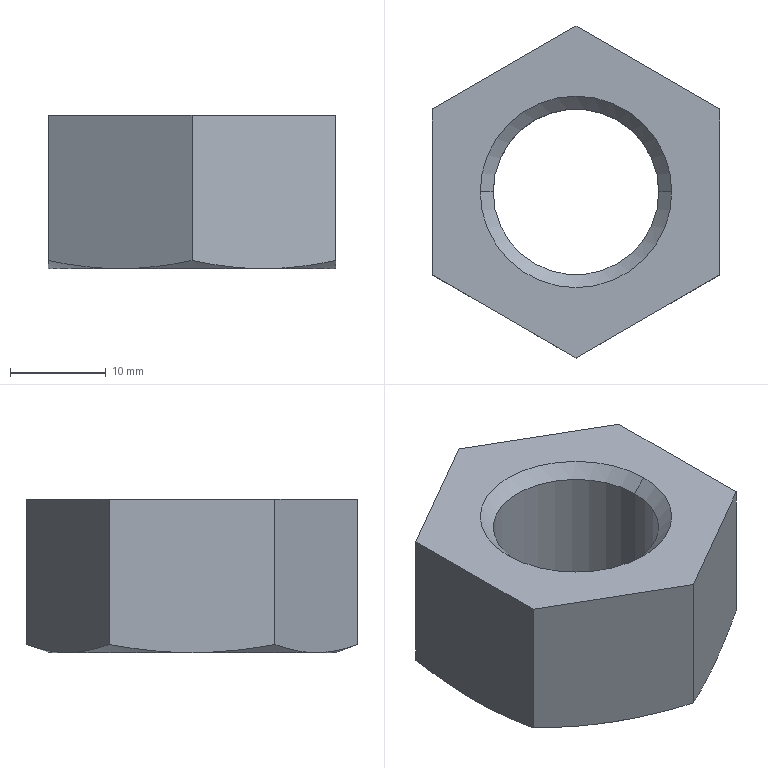Part | SolidWorks | features BaseBody 1 | 1 solid | 20 faces | box 30 x 34.641 x 16 mm | volume 8589 mm3 | cone 10 | plane 8 | cylinder 2 | commonest cylinder face diameters 17.294 x2
STEP:
#1=CARTESIAN_POINT('',(-8.647,0.,1.353));
#2=VERTEX_POINT('',#1);
#3=CARTESIAN_POINT('',(8.647,0.,1.353));
#4=VERTEX_POINT('',#3);
#5=CARTESIAN_POINT('',(0.,0.,1.353));
#6=DIRECTION('',(0.,0.,1.));
#7=DIRECTION('',(1.,0.,0.));
#8=AXIS2_PLACEMENT_3D('',#5,#6,#7);
#9=CIRCLE('',#8,8.647);
#10=EDGE_CURVE('',#2,#4,#9,.T.);
#11=ORIENTED_EDGE('',*,*,#10,.F.);
#12=CARTESIAN_POINT('',(-8.647,0.,14.647));
#13=VERTEX_POINT('',#12);
#14=CARTESIAN_POINT('',(-8.647,0.,0.));
#15=DIRECTION('',(0.,0.,1.));
#16=VECTOR('',#15,1000.);
#17=LINE('',#14,#16);
#18=EDGE_CURVE('',#2,#13,#17,.T.);
#19=ORIENTED_EDGE('',*,*,#18,.T.);
#20=CARTESIAN_POINT('',(8.647,0.,14.647));
#21=VERTEX_POINT('',#20);
#22=CARTESIAN_POINT('',(0.,0.,14.647));
#23=DIRECTION('',(0.,0.,-1.));
#24=DIRECTION('',(1.,0.,0.));
#25=AXIS2_PLACEMENT_3D('',#22,#23,#24);
#26=CIRCLE('',#25,8.647);
#27=EDGE_CURVE('',#21,#13,#26,.T.);
#28=ORIENTED_EDGE('',*,*,#27,.F.);
#29=CARTESIAN_POINT('',(8.647,0.,0.));
#30=DIRECTION('',(0.,0.,1.));
#31=VECTOR('',#30,1000.);
#32=LINE('',#29,#31);
#33=EDGE_CURVE('',#4,#21,#32,.T.);
#34=ORIENTED_EDGE('',*,*,#33,.F.);
#35=EDGE_LOOP('',(#11,#19,#28,#34));
#36=FACE_OUTER_BOUND('',#35,.T.);
#37=CARTESIAN_POINT('',(0.,0.,0.));
#38=DIRECTION('',(0.,0.,1.));
#39=DIRECTION('',(1.,0.,0.));
#40=AXIS2_PLACEMENT_3D('',#37,#38,#39);
#41=CYLINDRICAL_SURFACE('',#40,8.647);
#42=ADVANCED_FACE('',(#36),#41,.F.);
#43=ORIENTED_EDGE('',*,*,#27,.T.);
#44=CARTESIAN_POINT('',(-10.,0.,16.));
#45=VERTEX_POINT('',#44);
#46=CARTESIAN_POINT('',(-10.,0.,16.));
#47=DIRECTION('',(-0.7071,0.,0.7071));
#48=VECTOR('',#47,1000.);
#49=LINE('',#46,#48);
#50=EDGE_CURVE('',#13,#45,#49,.T.);
#51=ORIENTED_EDGE('',*,*,#50,.T.);
#52=CARTESIAN_POINT('',(10.,0.,16.));
#53=VERTEX_POINT('',#52);
#54=CARTESIAN_POINT('',(0.,0.,16.));
#55=DIRECTION('',(0.,0.,-1.));
#56=DIRECTION('',(1.,0.,0.));
#57=AXIS2_PLACEMENT_3D('',#54,#55,#56);
#58=CIRCLE('',#57,10.);
#59=EDGE_CURVE('',#53,#45,#58,.T.);
#60=ORIENTED_EDGE('',*,*,#59,.F.);
#61=CARTESIAN_POINT('',(10.,0.,16.));
#62=DIRECTION('',(0.7071,0.,0.7071));
#63=VECTOR('',#62,1000.);
#64=LINE('',#61,#63);
#65=EDGE_CURVE('',#21,#53,#64,.T.);
#66=ORIENTED_EDGE('',*,*,#65,.F.);
#67=EDGE_LOOP('',(#43,#51,#60,#66));
#68=FACE_OUTER_BOUND('',#67,.T.);
#69=CARTESIAN_POINT('',(0.,0.,16.));
#70=DIRECTION('',(0.,0.,1.));
#71=DIRECTION('',(1.,0.,0.));
#72=AXIS2_PLACEMENT_3D('',#69,#70,#71);
#73=CONICAL_SURFACE('',#72,10.,0.7854);
#74=ADVANCED_FACE('',(#68),#73,.F.);
#75=ORIENTED_EDGE('',*,*,#10,.T.);
#76=CARTESIAN_POINT('',(10.,0.,0.));
#77=VERTEX_POINT('',#76);
#78=CARTESIAN_POINT('',(10.,0.,0.));
#79=DIRECTION('',(0.7071,0.,-0.7071));
#80=VECTOR('',#79,1000.);
#81=LINE('',#78,#80);
#82=EDGE_CURVE('',#4,#77,#81,.T.);
#83=ORIENTED_EDGE('',*,*,#82,.T.);
#84=CARTESIAN_POINT('',(-10.,0.,0.));
#85=VERTEX_POINT('',#84);
#86=CARTESIAN_POINT('',(0.,0.,0.));
#87=DIRECTION('',(0.,0.,1.));
#88=DIRECTION('',(-1.,0.,0.));
#89=AXIS2_PLACEMENT_3D('',#86,#87,#88);
#90=CIRCLE('',#89,10.);
#91=EDGE_CURVE('',#85,#77,#90,.T.);
#92=ORIENTED_EDGE('',*,*,#91,.F.);
#93=CARTESIAN_POINT('',(-10.,0.,0.));
#94=DIRECTION('',(-0.7071,0.,-0.7071));
#95=VECTOR('',#94,1000.);
#96=LINE('',#93,#95);
#97=EDGE_CURVE('',#2,#85,#96,.T.);
#98=ORIENTED_EDGE('',*,*,#97,.F.);
#99=EDGE_LOOP('',(#75,#83,#92,#98));
#100=FACE_OUTER_BOUND('',#99,.T.);
#101=CARTESIAN_POINT('',(0.,0.,0.));
#102=DIRECTION('',(0.,0.,-1.));
#103=DIRECTION('',(-1.,0.,0.));
#104=AXIS2_PLACEMENT_3D('',#101,#102,#103);
#105=CONICAL_SURFACE('',#104,10.,0.7854);
#106=ADVANCED_FACE('',(#100),#105,.F.);
#107=ORIENTED_EDGE('',*,*,#18,.F.);
#108=CARTESIAN_POINT('',(0.,0.,1.353));
#109=DIRECTION('',(0.,0.,1.));
#110=DIRECTION('',(1.,0.,0.));
#111=AXIS2_PLACEMENT_3D('',#108,#109,#110);
#112=CIRCLE('',#111,8.647);
#113=EDGE_CURVE('',#4,#2,#112,.T.);
#114=ORIENTED_EDGE('',*,*,#113,.F.);
#115=ORIENTED_EDGE('',*,*,#33,.T.);
#116=CARTESIAN_POINT('',(0.,0.,14.647));
#117=DIRECTION('',(0.,0.,-1.));
#118=DIRECTION('',(1.,0.,0.));
#119=AXIS2_PLACEMENT_3D('',#116,#117,#118);
#120=CIRCLE('',#119,8.647);
#121=EDGE_CURVE('',#13,#21,#120,.T.);
#122=ORIENTED_EDGE('',*,*,#121,.F.);
#123=EDGE_LOOP('',(#107,#114,#115,#122));
#124=FACE_OUTER_BOUND('',#123,.T.);
#125=CARTESIAN_POINT('',(0.,0.,0.));
#126=DIRECTION('',(0.,0.,1.));
#127=DIRECTION('',(1.,0.,0.));
#128=AXIS2_PLACEMENT_3D('',#125,#126,#127);
#129=CYLINDRICAL_SURFACE('',#128,8.647);
#130=ADVANCED_FACE('',(#124),#129,.F.);
#131=ORIENTED_EDGE('',*,*,#50,.F.);
#132=ORIENTED_EDGE('',*,*,#121,.T.);
#133=ORIENTED_EDGE('',*,*,#65,.T.);
#134=CARTESIAN_POINT('',(0.,0.,16.));
#135=DIRECTION('',(0.,0.,-1.));
#136=DIRECTION('',(1.,0.,0.));
#137=AXIS2_PLACEMENT_3D('',#134,#135,#136);
#138=CIRCLE('',#137,10.);
#139=EDGE_CURVE('',#45,#53,#138,.T.);
#140=ORIENTED_EDGE('',*,*,#139,.F.);
#141=EDGE_LOOP('',(#131,#132,#133,#140));
#142=FACE_OUTER_BOUND('',#141,.T.);
#143=CARTESIAN_POINT('',(0.,0.,16.));
#144=DIRECTION('',(0.,0.,1.));
#145=DIRECTION('',(1.,0.,0.));
#146=AXIS2_PLACEMENT_3D('',#143,#144,#145);
#147=CONICAL_SURFACE('',#146,10.,0.7854);
#148=ADVANCED_FACE('',(#142),#147,.F.);
#149=ORIENTED_EDGE('',*,*,#82,.F.);
#150=ORIENTED_EDGE('',*,*,#113,.T.);
#151=ORIENTED_EDGE('',*,*,#97,.T.);
#152=CARTESIAN_POINT('',(0.,0.,0.));
#153=DIRECTION('',(0.,0.,1.));
#154=DIRECTION('',(-1.,0.,0.));
#155=AXIS2_PLACEMENT_3D('',#152,#153,#154);
#156=CIRCLE('',#155,10.);
#157=EDGE_CURVE('',#77,#85,#156,.T.);
#158=ORIENTED_EDGE('',*,*,#157,.F.);
#159=EDGE_LOOP('',(#149,#150,#151,#158));
#160=FACE_OUTER_BOUND('',#159,.T.);
#161=CARTESIAN_POINT('',(0.,0.,0.));
#162=DIRECTION('',(0.,0.,-1.));
#163=DIRECTION('',(-1.,0.,0.));
#164=AXIS2_PLACEMENT_3D('',#161,#162,#163);
#165=CONICAL_SURFACE('',#164,10.,0.7854);
#166=ADVANCED_FACE('',(#160),#165,.F.);
#167=ORIENTED_EDGE('',*,*,#59,.T.);
#168=ORIENTED_EDGE('',*,*,#139,.T.);
#169=EDGE_LOOP('',(#167,#168));
#170=FACE_BOUND('',#169,.T.);
#171=CARTESIAN_POINT('',(15.,-8.66,16.));
#172=VERTEX_POINT('',#171);
#173=CARTESIAN_POINT('',(15.,8.66,16.));
#174=VERTEX_POINT('',#173);
#175=CARTESIAN_POINT('',(15.,0.,16.));
#176=DIRECTION('',(0.,1.,0.));
#177=VECTOR('',#176,1000.);
#178=LINE('',#175,#177);
#179=EDGE_CURVE('',#172,#174,#178,.T.);
#180=ORIENTED_EDGE('',*,*,#179,.T.);
#181=CARTESIAN_POINT('',(0.,17.321,16.));
#182=VERTEX_POINT('',#181);
#183=CARTESIAN_POINT('',(15.,8.66,16.));
#184=DIRECTION('',(-0.866,0.5,0.));
#185=VECTOR('',#184,1000.);
#186=LINE('',#183,#185);
#187=EDGE_CURVE('',#174,#182,#186,.T.);
#188=ORIENTED_EDGE('',*,*,#187,.T.);
#189=CARTESIAN_POINT('',(-15.,8.66,16.));
#190=VERTEX_POINT('',#189);
#191=CARTESIAN_POINT('',(0.,17.321,16.));
#192=DIRECTION('',(-0.866,-0.5,0.));
#193=VECTOR('',#192,1000.);
#194=LINE('',#191,#193);
#195=EDGE_CURVE('',#182,#190,#194,.T.);
#196=ORIENTED_EDGE('',*,*,#195,.T.);
#197=CARTESIAN_POINT('',(-15.,-8.66,16.));
#198=VERTEX_POINT('',#197);
#199=CARTESIAN_POINT('',(-15.,0.,16.));
#200=DIRECTION('',(0.,-1.,0.));
#201=VECTOR('',#200,1000.);
#202=LINE('',#199,#201);
#203=EDGE_CURVE('',#190,#198,#202,.T.);
#204=ORIENTED_EDGE('',*,*,#203,.T.);
#205=CARTESIAN_POINT('',(0.,-17.321,16.));
#206=VERTEX_POINT('',#205);
#207=CARTESIAN_POINT('',(-15.,-8.66,16.));
#208=DIRECTION('',(0.866,-0.5,0.));
#209=VECTOR('',#208,1000.);
#210=LINE('',#207,#209);
#211=EDGE_CURVE('',#198,#206,#210,.T.);
#212=ORIENTED_EDGE('',*,*,#211,.T.);
#213=CARTESIAN_POINT('',(0.,-17.321,16.));
#214=DIRECTION('',(0.866,0.5,0.));
#215=VECTOR('',#214,1000.);
#216=LINE('',#213,#215);
#217=EDGE_CURVE('',#206,#172,#216,.T.);
#218=ORIENTED_EDGE('',*,*,#217,.T.);
#219=EDGE_LOOP('',(#180,#188,#196,#204,#212,#218));
#220=FACE_OUTER_BOUND('',#219,.T.);
#221=CARTESIAN_POINT('',(0.,0.,16.));
#222=DIRECTION('',(0.,0.,1.));
#223=DIRECTION('',(1.,0.,0.));
#224=AXIS2_PLACEMENT_3D('',#221,#222,#223);
#225=PLANE('',#224);
#226=ADVANCED_FACE('',(#170,#220),#225,.T.);
#227=ORIENTED_EDGE('',*,*,#91,.T.);
#228=ORIENTED_EDGE('',*,*,#157,.T.);
#229=EDGE_LOOP('',(#227,#228));
#230=FACE_BOUND('',#229,.T.);
#231=CARTESIAN_POINT('',(-7.5,-12.99,0.));
#232=VERTEX_POINT('',#231);
#233=CARTESIAN_POINT('',(7.5,-12.99,0.));
#234=VERTEX_POINT('',#233);
#235=CARTESIAN_POINT('',(0.,0.,0.));
#236=DIRECTION('',(0.,0.,1.));
#237=DIRECTION('',(1.,0.,0.));
#238=AXIS2_PLACEMENT_3D('',#235,#236,#237);
#239=CIRCLE('',#238,15.);
#240=EDGE_CURVE('',#232,#234,#239,.T.);
#241=ORIENTED_EDGE('',*,*,#240,.F.);
#242=CARTESIAN_POINT('',(-15.,0.,0.));
#243=VERTEX_POINT('',#242);
#244=CARTESIAN_POINT('',(0.,0.,0.));
#245=DIRECTION('',(0.,0.,1.));
#246=DIRECTION('',(0.,-1.,0.));
#247=AXIS2_PLACEMENT_3D('',#244,#245,#246);
#248=CIRCLE('',#247,15.);
#249=EDGE_CURVE('',#243,#232,#248,.T.);
#250=ORIENTED_EDGE('',*,*,#249,.F.);
#251=CARTESIAN_POINT('',(-7.5,12.99,0.));
#252=VERTEX_POINT('',#251);
#253=CARTESIAN_POINT('',(0.,0.,0.));
#254=DIRECTION('',(0.,0.,1.));
#255=DIRECTION('',(0.,-1.,0.));
#256=AXIS2_PLACEMENT_3D('',#253,#254,#255);
#257=CIRCLE('',#256,15.);
#258=EDGE_CURVE('',#252,#243,#257,.T.);
#259=ORIENTED_EDGE('',*,*,#258,.F.);
#260=CARTESIAN_POINT('',(7.5,12.99,0.));
#261=VERTEX_POINT('',#260);
#262=CARTESIAN_POINT('',(0.,0.,0.));
#263=DIRECTION('',(0.,0.,1.));
#264=DIRECTION('',(1.,0.,0.));
#265=AXIS2_PLACEMENT_3D('',#262,#263,#264);
#266=CIRCLE('',#265,15.);
#267=EDGE_CURVE('',#261,#252,#266,.T.);
#268=ORIENTED_EDGE('',*,*,#267,.F.);
#269=CARTESIAN_POINT('',(15.,0.,0.));
#270=VERTEX_POINT('',#269);
#271=CARTESIAN_POINT('',(0.,0.,0.));
#272=DIRECTION('',(0.,0.,1.));
#273=DIRECTION('',(0.,-1.,0.));
#274=AXIS2_PLACEMENT_3D('',#271,#272,#273);
#275=CIRCLE('',#274,15.);
#276=EDGE_CURVE('',#270,#261,#275,.T.);
#277=ORIENTED_EDGE('',*,*,#276,.F.);
#278=CARTESIAN_POINT('',(0.,0.,0.));
#279=DIRECTION('',(0.,0.,1.));
#280=DIRECTION('',(1.,0.,0.));
#281=AXIS2_PLACEMENT_3D('',#278,#279,#280);
#282=CIRCLE('',#281,15.);
#283=EDGE_CURVE('',#234,#270,#282,.T.);
#284=ORIENTED_EDGE('',*,*,#283,.F.);
#285=EDGE_LOOP('',(#241,#250,#259,#268,#277,#284));
#286=FACE_OUTER_BOUND('',#285,.T.);
#287=CARTESIAN_POINT('',(0.,0.,0.));
#288=DIRECTION('',(0.,0.,1.));
#289=DIRECTION('',(1.,0.,0.));
#290=AXIS2_PLACEMENT_3D('',#287,#288,#289);
#291=PLANE('',#290);
#292=ADVANCED_FACE('',(#230,#286),#291,.F.);
#293=CARTESIAN_POINT('',(15.,8.66,0.8446));
#294=VERTEX_POINT('',#293);
#295=CARTESIAN_POINT('',(7.5,12.99,0.));
#296=CARTESIAN_POINT('',(8.762,12.262,0.));
#297=CARTESIAN_POINT('',(10.017,11.537,0.07863));
#298=CARTESIAN_POINT('',(12.516,10.094,0.3711));
#299=CARTESIAN_POINT('',(13.76,9.376,0.584));
#300=CARTESIAN_POINT('',(15.,8.66,0.8446));
#301=B_SPLINE_CURVE_WITH_KNOTS('',3,(#295,#296,#297,#298,#299,#300),.UNSPECIFIED.,.F.,.F.,(4,2,4),(0.,0.004351,0.008701),.UNSPECIFIED.);
#302=EDGE_CURVE('',#261,#294,#301,.T.);
#303=ORIENTED_EDGE('',*,*,#302,.F.);
#304=CARTESIAN_POINT('',(0.,17.321,0.8446));
#305=VERTEX_POINT('',#304);
#306=CARTESIAN_POINT('',(0.,17.321,0.8446));
#307=CARTESIAN_POINT('',(1.24,16.605,0.584));
#308=CARTESIAN_POINT('',(2.484,15.886,0.3711));
#309=CARTESIAN_POINT('',(4.983,14.444,0.07863));
#310=CARTESIAN_POINT('',(6.238,13.719,0.));
#311=CARTESIAN_POINT('',(7.5,12.99,0.));
#312=B_SPLINE_CURVE_WITH_KNOTS('',3,(#306,#307,#308,#309,#310,#311),.UNSPECIFIED.,.F.,.F.,(4,2,4),(0.,0.004351,0.008701),.UNSPECIFIED.);
#313=EDGE_CURVE('',#305,#261,#312,.T.);
#314=ORIENTED_EDGE('',*,*,#313,.F.);
#315=CARTESIAN_POINT('',(0.,17.321,16.));
#316=DIRECTION('',(0.,0.,-1.));
#317=VECTOR('',#316,1000.);
#318=LINE('',#315,#317);
#319=EDGE_CURVE('',#182,#305,#318,.T.);
#320=ORIENTED_EDGE('',*,*,#319,.F.);
#321=ORIENTED_EDGE('',*,*,#187,.F.);
#322=CARTESIAN_POINT('',(15.,8.66,16.));
#323=DIRECTION('',(0.,0.,1.));
#324=VECTOR('',#323,1000.);
#325=LINE('',#322,#324);
#326=EDGE_CURVE('',#294,#174,#325,.T.);
#327=ORIENTED_EDGE('',*,*,#326,.F.);
#328=EDGE_LOOP('',(#303,#314,#320,#321,#327));
#329=FACE_OUTER_BOUND('',#328,.T.);
#330=CARTESIAN_POINT('',(15.,8.66,16.));
#331=DIRECTION('',(-0.5,-0.866,0.));
#332=DIRECTION('',(0.866,-0.5,0.));
#333=AXIS2_PLACEMENT_3D('',#330,#331,#332);
#334=PLANE('',#333);
#335=ADVANCED_FACE('',(#329),#334,.F.);
#336=CARTESIAN_POINT('',(15.,-8.66,0.8446));
#337=VERTEX_POINT('',#336);
#338=CARTESIAN_POINT('',(15.,0.,0.));
#339=CARTESIAN_POINT('',(15.,-1.457,0.));
#340=CARTESIAN_POINT('',(15.,-2.907,0.07863));
#341=CARTESIAN_POINT('',(15.,-5.792,0.3711));
#342=CARTESIAN_POINT('',(15.,-7.229,0.584));
#343=CARTESIAN_POINT('',(15.,-8.66,0.8446));
#344=B_SPLINE_CURVE_WITH_KNOTS('',3,(#338,#339,#340,#341,#342,#343),.UNSPECIFIED.,.F.,.F.,(4,2,4),(0.,0.004351,0.008701),.UNSPECIFIED.);
#345=EDGE_CURVE('',#270,#337,#344,.T.);
#346=ORIENTED_EDGE('',*,*,#345,.F.);
#347=CARTESIAN_POINT('',(15.,8.66,0.8446));
#348=CARTESIAN_POINT('',(15.,7.229,0.584));
#349=CARTESIAN_POINT('',(15.,5.792,0.3711));
#350=CARTESIAN_POINT('',(15.,2.907,0.07863));
#351=CARTESIAN_POINT('',(15.,1.457,0.));
#352=CARTESIAN_POINT('',(15.,0.,0.));
#353=B_SPLINE_CURVE_WITH_KNOTS('',3,(#347,#348,#349,#350,#351,#352),.UNSPECIFIED.,.F.,.F.,(4,2,4),(0.,0.004351,0.008701),.UNSPECIFIED.);
#354=EDGE_CURVE('',#294,#270,#353,.T.);
#355=ORIENTED_EDGE('',*,*,#354,.F.);
#356=ORIENTED_EDGE('',*,*,#326,.T.);
#357=ORIENTED_EDGE('',*,*,#179,.F.);
#358=CARTESIAN_POINT('',(15.,-8.66,16.));
#359=DIRECTION('',(0.,0.,1.));
#360=VECTOR('',#359,1000.);
#361=LINE('',#358,#360);
#362=EDGE_CURVE('',#337,#172,#361,.T.);
#363=ORIENTED_EDGE('',*,*,#362,.F.);
#364=EDGE_LOOP('',(#346,#355,#356,#357,#363));
#365=FACE_OUTER_BOUND('',#364,.T.);
#366=CARTESIAN_POINT('',(15.,-8.66,16.));
#367=DIRECTION('',(-1.,0.,0.));
#368=DIRECTION('',(0.,0.,1.));
#369=AXIS2_PLACEMENT_3D('',#366,#367,#368);
#370=PLANE('',#369);
#371=ADVANCED_FACE('',(#365),#370,.F.);
#372=CARTESIAN_POINT('',(0.,-17.321,0.8446));
#373=VERTEX_POINT('',#372);
#374=CARTESIAN_POINT('',(7.5,-12.99,0.));
#375=CARTESIAN_POINT('',(6.238,-13.719,0.));
#376=CARTESIAN_POINT('',(4.983,-14.444,0.07863));
#377=CARTESIAN_POINT('',(2.484,-15.886,0.3711));
#378=CARTESIAN_POINT('',(1.24,-16.605,0.584));
#379=CARTESIAN_POINT('',(0.,-17.321,0.8446));
#380=B_SPLINE_CURVE_WITH_KNOTS('',3,(#374,#375,#376,#377,#378,#379),.UNSPECIFIED.,.F.,.F.,(4,2,4),(0.,0.004351,0.008701),.UNSPECIFIED.);
#381=EDGE_CURVE('',#234,#373,#380,.T.);
#382=ORIENTED_EDGE('',*,*,#381,.F.);
#383=CARTESIAN_POINT('',(15.,-8.66,0.8446));
#384=CARTESIAN_POINT('',(13.76,-9.376,0.584));
#385=CARTESIAN_POINT('',(12.516,-10.094,0.3711));
#386=CARTESIAN_POINT('',(10.017,-11.537,0.07863));
#387=CARTESIAN_POINT('',(8.762,-12.262,0.));
#388=CARTESIAN_POINT('',(7.5,-12.99,0.));
#389=B_SPLINE_CURVE_WITH_KNOTS('',3,(#383,#384,#385,#386,#387,#388),.UNSPECIFIED.,.F.,.F.,(4,2,4),(0.,0.004351,0.008701),.UNSPECIFIED.);
#390=EDGE_CURVE('',#337,#234,#389,.T.);
#391=ORIENTED_EDGE('',*,*,#390,.F.);
#392=ORIENTED_EDGE('',*,*,#362,.T.);
#393=ORIENTED_EDGE('',*,*,#217,.F.);
#394=CARTESIAN_POINT('',(0.,-17.321,16.));
#395=DIRECTION('',(0.,0.,1.));
#396=VECTOR('',#395,1000.);
#397=LINE('',#394,#396);
#398=EDGE_CURVE('',#373,#206,#397,.T.);
#399=ORIENTED_EDGE('',*,*,#398,.F.);
#400=EDGE_LOOP('',(#382,#391,#392,#393,#399));
#401=FACE_OUTER_BOUND('',#400,.T.);
#402=CARTESIAN_POINT('',(0.,-17.321,16.));
#403=DIRECTION('',(-0.5,0.866,0.));
#404=DIRECTION('',(-0.866,-0.5,0.));
#405=AXIS2_PLACEMENT_3D('',#402,#403,#404);
#406=PLANE('',#405);
#407=ADVANCED_FACE('',(#401),#406,.F.);
#408=CARTESIAN_POINT('',(-15.,-8.66,0.8446));
#409=VERTEX_POINT('',#408);
#410=CARTESIAN_POINT('',(-7.5,-12.99,0.));
#411=CARTESIAN_POINT('',(-8.762,-12.262,0.));
#412=CARTESIAN_POINT('',(-10.017,-11.537,0.07863));
#413=CARTESIAN_POINT('',(-12.516,-10.094,0.3711));
#414=CARTESIAN_POINT('',(-13.76,-9.376,0.584));
#415=CARTESIAN_POINT('',(-15.,-8.66,0.8446));
#416=B_SPLINE_CURVE_WITH_KNOTS('',3,(#410,#411,#412,#413,#414,#415),.UNSPECIFIED.,.F.,.F.,(4,2,4),(0.,0.004351,0.008701),.UNSPECIFIED.);
#417=EDGE_CURVE('',#232,#409,#416,.T.);
#418=ORIENTED_EDGE('',*,*,#417,.F.);
#419=CARTESIAN_POINT('',(0.,-17.321,0.8446));
#420=CARTESIAN_POINT('',(-1.24,-16.605,0.584));
#421=CARTESIAN_POINT('',(-2.484,-15.886,0.3711));
#422=CARTESIAN_POINT('',(-4.983,-14.444,0.07863));
#423=CARTESIAN_POINT('',(-6.238,-13.719,0.));
#424=CARTESIAN_POINT('',(-7.5,-12.99,0.));
#425=B_SPLINE_CURVE_WITH_KNOTS('',3,(#419,#420,#421,#422,#423,#424),.UNSPECIFIED.,.F.,.F.,(4,2,4),(0.,0.004351,0.008701),.UNSPECIFIED.);
#426=EDGE_CURVE('',#373,#232,#425,.T.);
#427=ORIENTED_EDGE('',*,*,#426,.F.);
#428=ORIENTED_EDGE('',*,*,#398,.T.);
#429=ORIENTED_EDGE('',*,*,#211,.F.);
#430=CARTESIAN_POINT('',(-15.,-8.66,16.));
#431=DIRECTION('',(0.,0.,1.));
#432=VECTOR('',#431,1000.);
#433=LINE('',#430,#432);
#434=EDGE_CURVE('',#409,#198,#433,.T.);
#435=ORIENTED_EDGE('',*,*,#434,.F.);
#436=EDGE_LOOP('',(#418,#427,#428,#429,#435));
#437=FACE_OUTER_BOUND('',#436,.T.);
#438=CARTESIAN_POINT('',(-15.,-8.66,16.));
#439=DIRECTION('',(0.5,0.866,0.));
#440=DIRECTION('',(-0.866,0.5,0.));
#441=AXIS2_PLACEMENT_3D('',#438,#439,#440);
#442=PLANE('',#441);
#443=ADVANCED_FACE('',(#437),#442,.F.);
#444=CARTESIAN_POINT('',(-15.,8.66,0.8446));
#445=VERTEX_POINT('',#444);
#446=CARTESIAN_POINT('',(-15.,0.,0.));
#447=CARTESIAN_POINT('',(-15.,1.457,0.));
#448=CARTESIAN_POINT('',(-15.,2.907,0.07863));
#449=CARTESIAN_POINT('',(-15.,5.792,0.3711));
#450=CARTESIAN_POINT('',(-15.,7.229,0.584));
#451=CARTESIAN_POINT('',(-15.,8.66,0.8446));
#452=B_SPLINE_CURVE_WITH_KNOTS('',3,(#446,#447,#448,#449,#450,#451),.UNSPECIFIED.,.F.,.F.,(4,2,4),(0.,0.004351,0.008701),.UNSPECIFIED.);
#453=EDGE_CURVE('',#243,#445,#452,.T.);
#454=ORIENTED_EDGE('',*,*,#453,.F.);
#455=CARTESIAN_POINT('',(-15.,-8.66,0.8446));
#456=CARTESIAN_POINT('',(-15.,-7.229,0.584));
#457=CARTESIAN_POINT('',(-15.,-5.792,0.3711));
#458=CARTESIAN_POINT('',(-15.,-2.907,0.07863));
#459=CARTESIAN_POINT('',(-15.,-1.457,0.));
#460=CARTESIAN_POINT('',(-15.,0.,0.));
#461=B_SPLINE_CURVE_WITH_KNOTS('',3,(#455,#456,#457,#458,#459,#460),.UNSPECIFIED.,.F.,.F.,(4,2,4),(0.,0.004351,0.008701),.UNSPECIFIED.);
#462=EDGE_CURVE('',#409,#243,#461,.T.);
#463=ORIENTED_EDGE('',*,*,#462,.F.);
#464=ORIENTED_EDGE('',*,*,#434,.T.);
#465=ORIENTED_EDGE('',*,*,#203,.F.);
#466=CARTESIAN_POINT('',(-15.,8.66,16.));
#467=DIRECTION('',(0.,0.,1.));
#468=VECTOR('',#467,1000.);
#469=LINE('',#466,#468);
#470=EDGE_CURVE('',#445,#190,#469,.T.);
#471=ORIENTED_EDGE('',*,*,#470,.F.);
#472=EDGE_LOOP('',(#454,#463,#464,#465,#471));
#473=FACE_OUTER_BOUND('',#472,.T.);
#474=CARTESIAN_POINT('',(-15.,8.66,16.));
#475=DIRECTION('',(1.,0.,0.));
#476=DIRECTION('',(0.,0.,-1.));
#477=AXIS2_PLACEMENT_3D('',#474,#475,#476);
#478=PLANE('',#477);
#479=ADVANCED_FACE('',(#473),#478,.F.);
#480=CARTESIAN_POINT('',(-7.5,12.99,0.));
#481=CARTESIAN_POINT('',(-6.238,13.719,0.));
#482=CARTESIAN_POINT('',(-4.983,14.444,0.07863));
#483=CARTESIAN_POINT('',(-2.484,15.886,0.3711));
#484=CARTESIAN_POINT('',(-1.24,16.605,0.584));
#485=CARTESIAN_POINT('',(0.,17.321,0.8446));
#486=B_SPLINE_CURVE_WITH_KNOTS('',3,(#480,#481,#482,#483,#484,#485),.UNSPECIFIED.,.F.,.F.,(4,2,4),(0.,0.004351,0.008701),.UNSPECIFIED.);
#487=EDGE_CURVE('',#252,#305,#486,.T.);
#488=ORIENTED_EDGE('',*,*,#487,.F.);
#489=CARTESIAN_POINT('',(-15.,8.66,0.8446));
#490=CARTESIAN_POINT('',(-13.76,9.376,0.584));
#491=CARTESIAN_POINT('',(-12.516,10.094,0.3711));
#492=CARTESIAN_POINT('',(-10.017,11.537,0.07863));
#493=CARTESIAN_POINT('',(-8.762,12.262,0.));
#494=CARTESIAN_POINT('',(-7.5,12.99,0.));
#495=B_SPLINE_CURVE_WITH_KNOTS('',3,(#489,#490,#491,#492,#493,#494),.UNSPECIFIED.,.F.,.F.,(4,2,4),(0.,0.004351,0.008701),.UNSPECIFIED.);
#496=EDGE_CURVE('',#445,#252,#495,.T.);
#497=ORIENTED_EDGE('',*,*,#496,.F.);
#498=ORIENTED_EDGE('',*,*,#470,.T.);
#499=ORIENTED_EDGE('',*,*,#195,.F.);
#500=ORIENTED_EDGE('',*,*,#319,.T.);
#501=EDGE_LOOP('',(#488,#497,#498,#499,#500));
#502=FACE_OUTER_BOUND('',#501,.T.);
#503=CARTESIAN_POINT('',(0.,17.321,16.));
#504=DIRECTION('',(0.5,-0.866,0.));
#505=DIRECTION('',(0.866,0.5,0.));
#506=AXIS2_PLACEMENT_3D('',#503,#504,#505);
#507=PLANE('',#506);
#508=ADVANCED_FACE('',(#502),#507,.F.);
#509=ORIENTED_EDGE('',*,*,#345,.T.);
#510=ORIENTED_EDGE('',*,*,#390,.T.);
#511=ORIENTED_EDGE('',*,*,#283,.T.);
#512=EDGE_LOOP('',(#509,#510,#511));
#513=FACE_OUTER_BOUND('',#512,.T.);
#514=CARTESIAN_POINT('',(0.,0.,0.8497));
#515=DIRECTION('',(0.,0.,1.));
#516=DIRECTION('',(1.,0.,0.));
#517=AXIS2_PLACEMENT_3D('',#514,#515,#516);
#518=CONICAL_SURFACE('',#517,17.334,1.222);
#519=ADVANCED_FACE('',(#513),#518,.T.);
#520=ORIENTED_EDGE('',*,*,#381,.T.);
#521=ORIENTED_EDGE('',*,*,#426,.T.);
#522=ORIENTED_EDGE('',*,*,#240,.T.);
#523=EDGE_LOOP('',(#520,#521,#522));
#524=FACE_OUTER_BOUND('',#523,.T.);
#525=CARTESIAN_POINT('',(0.,0.,0.8497));
#526=DIRECTION('',(0.,0.,1.));
#527=DIRECTION('',(1.,0.,0.));
#528=AXIS2_PLACEMENT_3D('',#525,#526,#527);
#529=CONICAL_SURFACE('',#528,17.334,1.222);
#530=ADVANCED_FACE('',(#524),#529,.T.);
#531=ORIENTED_EDGE('',*,*,#417,.T.);
#532=ORIENTED_EDGE('',*,*,#462,.T.);
#533=ORIENTED_EDGE('',*,*,#249,.T.);
#534=EDGE_LOOP('',(#531,#532,#533));
#535=FACE_OUTER_BOUND('',#534,.T.);
#536=CARTESIAN_POINT('',(0.,0.,0.8497));
#537=DIRECTION('',(0.,0.,1.));
#538=DIRECTION('',(0.,-1.,0.));
#539=AXIS2_PLACEMENT_3D('',#536,#537,#538);
#540=CONICAL_SURFACE('',#539,17.334,1.222);
#541=ADVANCED_FACE('',(#535),#540,.T.);
#542=ORIENTED_EDGE('',*,*,#453,.T.);
#543=ORIENTED_EDGE('',*,*,#496,.T.);
#544=ORIENTED_EDGE('',*,*,#258,.T.);
#545=EDGE_LOOP('',(#542,#543,#544));
#546=FACE_OUTER_BOUND('',#545,.T.);
#547=CARTESIAN_POINT('',(0.,0.,0.8497));
#548=DIRECTION('',(0.,0.,1.));
#549=DIRECTION('',(0.,-1.,0.));
#550=AXIS2_PLACEMENT_3D('',#547,#548,#549);
#551=CONICAL_SURFACE('',#550,17.334,1.222);
#552=ADVANCED_FACE('',(#546),#551,.T.);
#553=ORIENTED_EDGE('',*,*,#313,.T.);
#554=ORIENTED_EDGE('',*,*,#267,.T.);
#555=ORIENTED_EDGE('',*,*,#487,.T.);
#556=EDGE_LOOP('',(#553,#554,#555));
#557=FACE_OUTER_BOUND('',#556,.T.);
#558=CARTESIAN_POINT('',(0.,0.,0.8497));
#559=DIRECTION('',(0.,0.,1.));
#560=DIRECTION('',(1.,0.,0.));
#561=AXIS2_PLACEMENT_3D('',#558,#559,#560);
#562=CONICAL_SURFACE('',#561,17.334,1.222);
#563=ADVANCED_FACE('',(#557),#562,.T.);
#564=ORIENTED_EDGE('',*,*,#302,.T.);
#565=ORIENTED_EDGE('',*,*,#354,.T.);
#566=ORIENTED_EDGE('',*,*,#276,.T.);
#567=EDGE_LOOP('',(#564,#565,#566));
#568=FACE_OUTER_BOUND('',#567,.T.);
#569=CARTESIAN_POINT('',(0.,0.,0.8497));
#570=DIRECTION('',(0.,0.,1.));
#571=DIRECTION('',(0.,-1.,0.));
#572=AXIS2_PLACEMENT_3D('',#569,#570,#571);
#573=CONICAL_SURFACE('',#572,17.334,1.222);
#574=ADVANCED_FACE('',(#568),#573,.T.);
#575=CLOSED_SHELL('',(#42,#74,#106,#130,#148,#166,#226,#292,#335,#371,#407,#443,#479,#508,#519,#530,#541,#552,#563,#574));
#576=MANIFOLD_SOLID_BREP('',#575);
#577=CARTESIAN_POINT('',(0.,0.,0.));
#578=DIRECTION('',(0.,0.,1.));
#579=DIRECTION('',(1.,0.,0.));
#580=AXIS2_PLACEMENT_3D('',#577,#578,#579);
#581=(LENGTH_UNIT()NAMED_UNIT(*)SI_UNIT(.MILLI.,.METRE.));
#582=UNCERTAINTY_MEASURE_WITH_UNIT(LENGTH_MEASURE(0.00001),#581,'','');
#583=(NAMED_UNIT(*)PLANE_ANGLE_UNIT()SI_UNIT($,.RADIAN.));
#584=(NAMED_UNIT(*)SI_UNIT($,.STERADIAN.)SOLID_ANGLE_UNIT());
#585=(GEOMETRIC_REPRESENTATION_CONTEXT(3)GLOBAL_UNCERTAINTY_ASSIGNED_CONTEXT((#582))GLOBAL_UNIT_ASSIGNED_CONTEXT((#581,#583,#584))REPRESENTATION_CONTEXT('',''));
#586=ADVANCED_BREP_SHAPE_REPRESENTATION('',(#576,#580),#585);